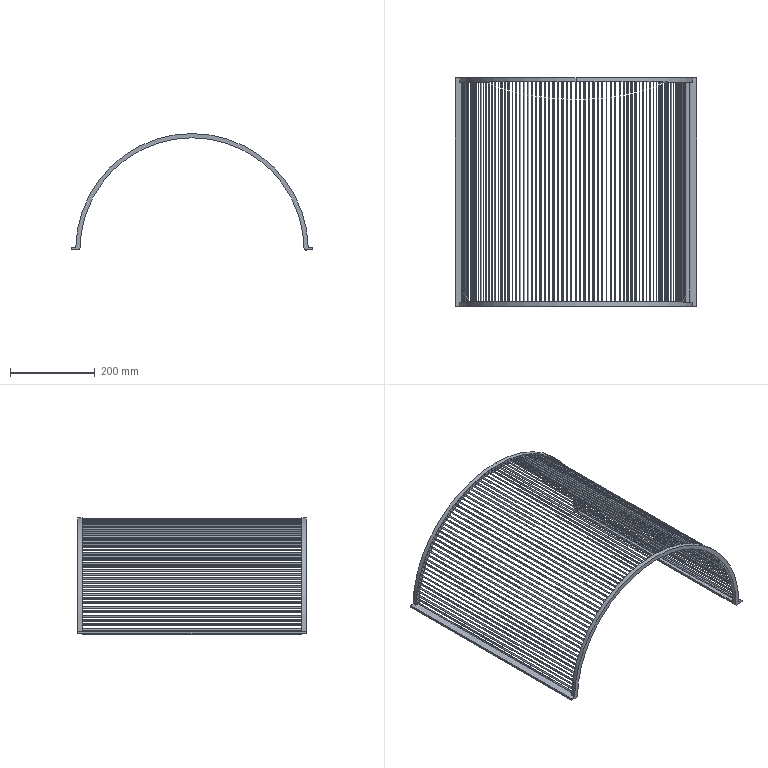Part | SolidWorks | features ICE 2, MirrorPattern 2, CirPattern 1, Extrusion 1, RefAxis 1 | 1 solid | 180 faces | box 570 x 540 x 276.117 mm | volume 657758 mm3 | cylinder 166 | plane 14 | commonest cylinder face diameters 3.435 x160 530 x3 550 x3